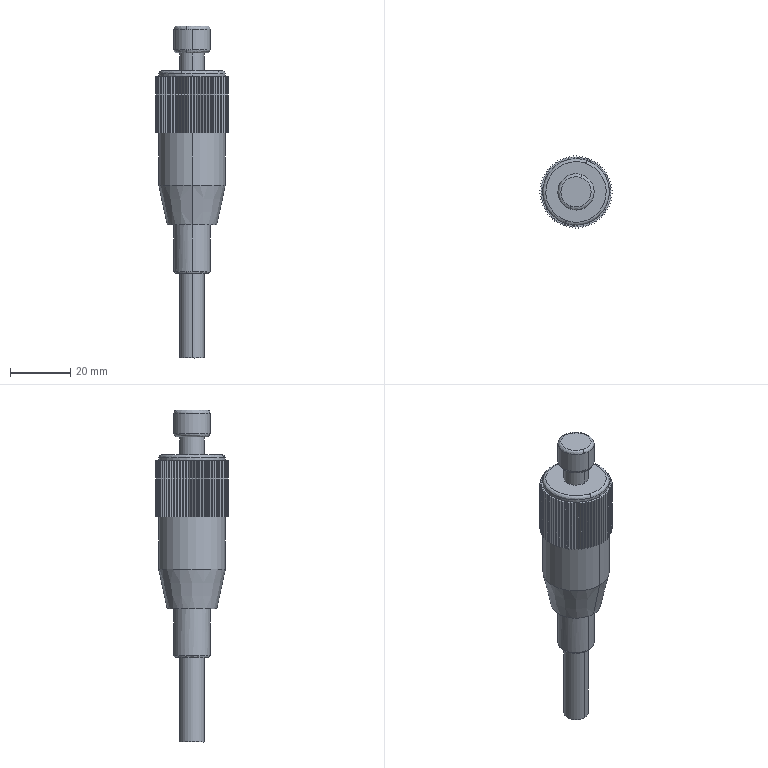Part | SolidWorks | features BaseBody 1 | 1 solid | 242 faces | box 23.853 x 23.868 x 109.775 mm | volume 23598 mm3 | plane 150 | cylinder 82 | spline 8 | cone 2 | commonest cylinder face diameters 23 x70 8 x4 12 x4 22 x4